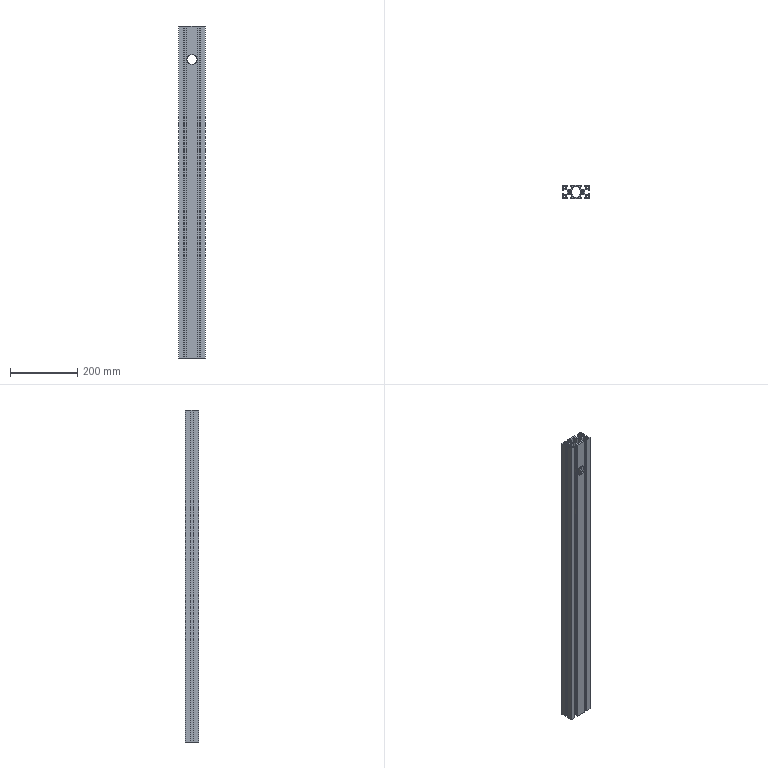Part | NX | 1 solid | 109 faces | box 80 x 40 x 991 mm | volume 1191942 mm3 | plane 94 | cylinder 15 | commonest cylinder face diameters 6 x8 8 x4 6.75 x2 30 x1